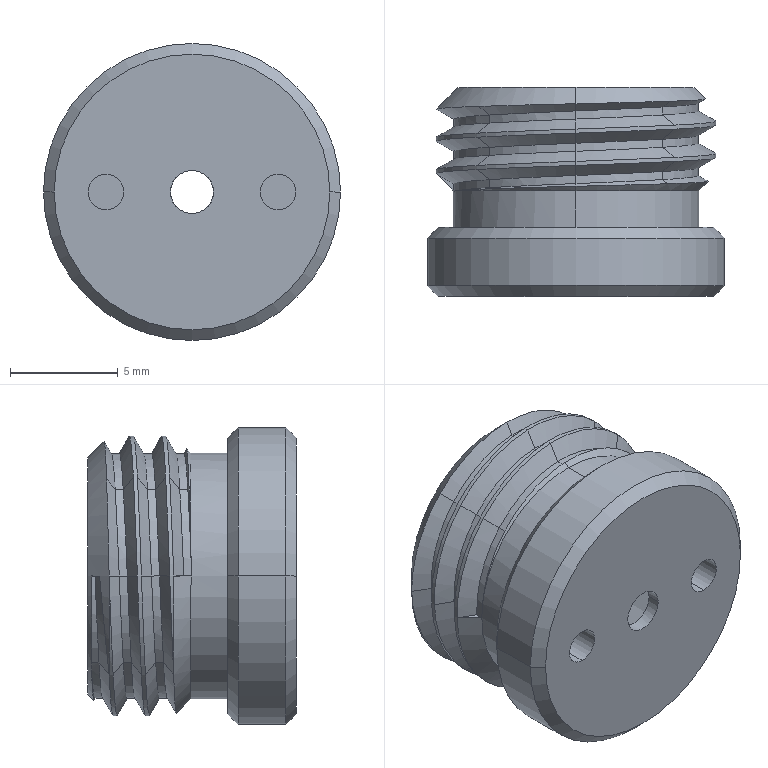Part | NX | features BREP 1 | 1 solid | 106 faces | box 13.8 x 9.7 x 13.8 mm | volume 672.716 mm3 | spline 48 | cylinder 40 | cone 11 | plane 7 | commonest cylinder face diameters 11.376 x23 13 x5 1.65 x4 2 x2 9 x2 11.4 x2